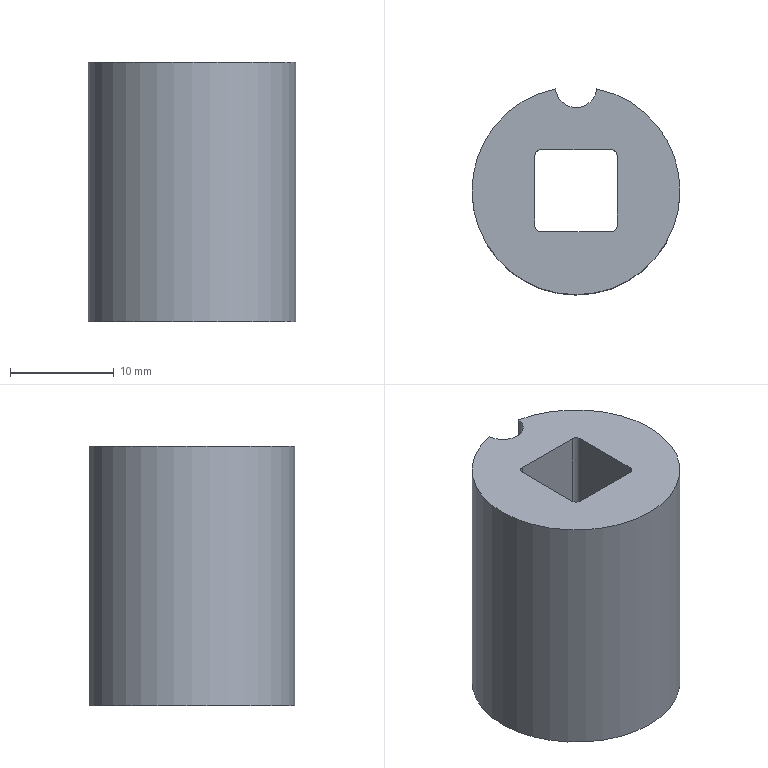Part | NX | features solid 2 | 1 solid | 14 faces | box 20 x 19.801 x 25 mm | volume 5087 mm3 | cylinder 7 | plane 7 | commonest cylinder face diameters 1.1 x4 4 x1 12.6 x1 20 x1
STEP:
#1=CARTESIAN_POINT('',(-371.503,508.125,-39.));
#2=VERTEX_POINT('',#1);
#3=CARTESIAN_POINT('',(-371.503,508.125,-14.));
#4=VERTEX_POINT('',#3);
#5=CARTESIAN_POINT('',(-371.503,508.125,-26.5));
#6=DIRECTION('',(0.,0.,1.));
#7=VECTOR('',#6,1000.);
#8=LINE('',#5,#7);
#9=EDGE_CURVE('',#2,#4,#8,.T.);
#10=ORIENTED_EDGE('',*,*,#9,.T.);
#11=CARTESIAN_POINT('',(-375.483,508.127,-14.));
#12=VERTEX_POINT('',#11);
#13=CARTESIAN_POINT('',(-373.499,498.326,-14.));
#14=DIRECTION('',(0.,0.,-1.));
#15=DIRECTION('',(0.000611,1.,0.));
#16=AXIS2_PLACEMENT_3D('',#13,#14,#15);
#17=CIRCLE('',#16,10.);
#18=EDGE_CURVE('',#4,#12,#17,.T.);
#19=ORIENTED_EDGE('',*,*,#18,.T.);
#20=CARTESIAN_POINT('',(-375.483,508.127,-39.));
#21=VERTEX_POINT('',#20);
#22=CARTESIAN_POINT('',(-375.483,508.127,-26.5));
#23=DIRECTION('',(0.,0.,1.));
#24=VECTOR('',#23,1000.);
#25=LINE('',#22,#24);
#26=EDGE_CURVE('',#12,#21,#25,.F.);
#27=ORIENTED_EDGE('',*,*,#26,.T.);
#28=CARTESIAN_POINT('',(-373.499,498.326,-39.));
#29=DIRECTION('',(0.,0.,-1.));
#30=DIRECTION('',(0.000611,1.,0.));
#31=AXIS2_PLACEMENT_3D('',#28,#29,#30);
#32=CIRCLE('',#31,10.);
#33=EDGE_CURVE('',#2,#21,#32,.T.);
#34=ORIENTED_EDGE('',*,*,#33,.F.);
#35=EDGE_LOOP('',(#10,#19,#27,#34));
#36=FACE_BOUND('',#35,.T.);
#37=CARTESIAN_POINT('',(-373.499,498.326,-39.));
#38=DIRECTION('',(0.,0.,1.));
#39=DIRECTION('',(0.000611,1.,0.));
#40=AXIS2_PLACEMENT_3D('',#37,#38,#39);
#41=CYLINDRICAL_SURFACE('',#40,10.);
#42=ADVANCED_FACE('',(#36),#41,.T.);
#43=CARTESIAN_POINT('',(-373.495,504.626,-39.));
#44=VERTEX_POINT('',#43);
#45=CARTESIAN_POINT('',(-373.499,498.326,-39.));
#46=DIRECTION('',(0.,0.,-1.));
#47=DIRECTION('',(0.000611,1.,0.));
#48=AXIS2_PLACEMENT_3D('',#45,#46,#47);
#49=CIRCLE('',#48,6.3);
#50=EDGE_CURVE('',#44,#44,#49,.T.);
#51=ORIENTED_EDGE('',*,*,#50,.F.);
#52=EDGE_LOOP('',(#51));
#53=FACE_BOUND('',#52,.T.);
#54=ORIENTED_EDGE('',*,*,#33,.T.);
#55=CARTESIAN_POINT('',(-373.493,508.326,-39.));
#56=DIRECTION('',(0.,0.,-1.));
#57=DIRECTION('',(0.000611,1.,0.));
#58=AXIS2_PLACEMENT_3D('',#55,#56,#57);
#59=CIRCLE('',#58,2.);
#60=EDGE_CURVE('',#2,#21,#59,.T.);
#61=ORIENTED_EDGE('',*,*,#60,.F.);
#62=EDGE_LOOP('',(#54,#61));
#63=FACE_BOUND('',#62,.T.);
#64=CARTESIAN_POINT('',(-373.499,498.326,-39.));
#65=DIRECTION('',(0.,0.,1.));
#66=DIRECTION('',(0.000611,1.,0.));
#67=AXIS2_PLACEMENT_3D('',#64,#65,#66);
#68=PLANE('',#67);
#69=ADVANCED_FACE('',(#53,#63),#68,.F.);
#70=CARTESIAN_POINT('',(-370.102,494.374,-14.));
#71=VERTEX_POINT('',#70);
#72=CARTESIAN_POINT('',(-376.902,494.378,-14.));
#73=VERTEX_POINT('',#72);
#74=CARTESIAN_POINT('',(-369.552,494.374,-14.));
#75=DIRECTION('',(-1.,0.000611,0.));
#76=VECTOR('',#75,1000.);
#77=LINE('',#74,#76);
#78=EDGE_CURVE('',#71,#73,#77,.T.);
#79=ORIENTED_EDGE('',*,*,#78,.T.);
#80=CARTESIAN_POINT('',(-377.451,494.928,-14.));
#81=VERTEX_POINT('',#80);
#82=CARTESIAN_POINT('',(-376.901,494.928,-14.));
#83=DIRECTION('',(0.,0.,-1.));
#84=DIRECTION('',(0.000611,1.,0.));
#85=AXIS2_PLACEMENT_3D('',#82,#83,#84);
#86=CIRCLE('',#85,0.55);
#87=EDGE_CURVE('',#81,#73,#86,.F.);
#88=ORIENTED_EDGE('',*,*,#87,.F.);
#89=CARTESIAN_POINT('',(-377.447,501.728,-14.));
#90=VERTEX_POINT('',#89);
#91=CARTESIAN_POINT('',(-377.452,494.378,-14.));
#92=DIRECTION('',(0.000611,1.,0.));
#93=VECTOR('',#92,1000.);
#94=LINE('',#91,#93);
#95=EDGE_CURVE('',#81,#90,#94,.T.);
#96=ORIENTED_EDGE('',*,*,#95,.T.);
#97=CARTESIAN_POINT('',(-376.897,502.278,-14.));
#98=VERTEX_POINT('',#97);
#99=CARTESIAN_POINT('',(-376.897,501.728,-14.));
#100=DIRECTION('',(0.,0.,-1.));
#101=DIRECTION('',(0.000611,1.,0.));
#102=AXIS2_PLACEMENT_3D('',#99,#100,#101);
#103=CIRCLE('',#102,0.55);
#104=EDGE_CURVE('',#98,#90,#103,.F.);
#105=ORIENTED_EDGE('',*,*,#104,.F.);
#106=CARTESIAN_POINT('',(-370.097,502.274,-14.));
#107=VERTEX_POINT('',#106);
#108=CARTESIAN_POINT('',(-369.547,502.274,-14.));
#109=DIRECTION('',(-1.,0.000611,0.));
#110=VECTOR('',#109,1000.);
#111=LINE('',#108,#110);
#112=EDGE_CURVE('',#107,#98,#111,.T.);
#113=ORIENTED_EDGE('',*,*,#112,.F.);
#114=CARTESIAN_POINT('',(-369.547,501.724,-14.));
#115=VERTEX_POINT('',#114);
#116=CARTESIAN_POINT('',(-370.097,501.724,-14.));
#117=DIRECTION('',(0.,0.,-1.));
#118=DIRECTION('',(0.000611,1.,0.));
#119=AXIS2_PLACEMENT_3D('',#116,#117,#118);
#120=CIRCLE('',#119,0.55);
#121=EDGE_CURVE('',#115,#107,#120,.F.);
#122=ORIENTED_EDGE('',*,*,#121,.F.);
#123=CARTESIAN_POINT('',(-369.551,494.924,-14.));
#124=VERTEX_POINT('',#123);
#125=CARTESIAN_POINT('',(-369.547,502.274,-14.));
#126=DIRECTION('',(-0.000611,-1.,0.));
#127=VECTOR('',#126,1000.);
#128=LINE('',#125,#127);
#129=EDGE_CURVE('',#115,#124,#128,.T.);
#130=ORIENTED_EDGE('',*,*,#129,.T.);
#131=CARTESIAN_POINT('',(-370.101,494.924,-14.));
#132=DIRECTION('',(0.,0.,-1.));
#133=DIRECTION('',(0.000611,1.,0.));
#134=AXIS2_PLACEMENT_3D('',#131,#132,#133);
#135=CIRCLE('',#134,0.55);
#136=EDGE_CURVE('',#71,#124,#135,.F.);
#137=ORIENTED_EDGE('',*,*,#136,.F.);
#138=EDGE_LOOP('',(#79,#88,#96,#105,#113,#122,#130,#137));
#139=FACE_BOUND('',#138,.T.);
#140=CARTESIAN_POINT('',(-373.493,508.326,-14.));
#141=DIRECTION('',(0.,0.,-1.));
#142=DIRECTION('',(0.000611,1.,0.));
#143=AXIS2_PLACEMENT_3D('',#140,#141,#142);
#144=CIRCLE('',#143,2.);
#145=EDGE_CURVE('',#4,#12,#144,.T.);
#146=ORIENTED_EDGE('',*,*,#145,.T.);
#147=ORIENTED_EDGE('',*,*,#18,.F.);
#148=EDGE_LOOP('',(#146,#147));
#149=FACE_BOUND('',#148,.T.);
#150=CARTESIAN_POINT('',(-373.499,498.326,-14.));
#151=DIRECTION('',(0.,0.,1.));
#152=DIRECTION('',(0.000611,1.,0.));
#153=AXIS2_PLACEMENT_3D('',#150,#151,#152);
#154=PLANE('',#153);
#155=ADVANCED_FACE('',(#139,#149),#154,.T.);
#156=ORIENTED_EDGE('',*,*,#50,.T.);
#157=EDGE_LOOP('',(#156));
#158=FACE_BOUND('',#157,.T.);
#159=CARTESIAN_POINT('',(-373.495,504.626,-22.));
#160=VERTEX_POINT('',#159);
#161=CARTESIAN_POINT('',(-373.499,498.326,-22.));
#162=DIRECTION('',(0.,0.,-1.));
#163=DIRECTION('',(0.000611,1.,0.));
#164=AXIS2_PLACEMENT_3D('',#161,#162,#163);
#165=CIRCLE('',#164,6.3);
#166=EDGE_CURVE('',#160,#160,#165,.T.);
#167=ORIENTED_EDGE('',*,*,#166,.F.);
#168=EDGE_LOOP('',(#167));
#169=FACE_BOUND('',#168,.T.);
#170=CARTESIAN_POINT('',(-373.499,498.326,-39.));
#171=DIRECTION('',(0.,0.,1.));
#172=DIRECTION('',(0.000611,1.,0.));
#173=AXIS2_PLACEMENT_3D('',#170,#171,#172);
#174=CYLINDRICAL_SURFACE('',#173,6.3);
#175=ADVANCED_FACE('',(#158,#169),#174,.F.);
#176=CARTESIAN_POINT('',(-370.097,502.274,-22.));
#177=VERTEX_POINT('',#176);
#178=CARTESIAN_POINT('',(-376.897,502.278,-22.));
#179=VERTEX_POINT('',#178);
#180=CARTESIAN_POINT('',(-373.497,502.276,-22.));
#181=DIRECTION('',(-1.,0.000611,0.));
#182=VECTOR('',#181,1000.);
#183=LINE('',#180,#182);
#184=EDGE_CURVE('',#177,#179,#183,.T.);
#185=ORIENTED_EDGE('',*,*,#184,.T.);
#186=CARTESIAN_POINT('',(-377.447,501.728,-22.));
#187=VERTEX_POINT('',#186);
#188=CARTESIAN_POINT('',(-376.897,501.728,-22.));
#189=DIRECTION('',(0.,0.,-1.));
#190=DIRECTION('',(0.000611,1.,0.));
#191=AXIS2_PLACEMENT_3D('',#188,#189,#190);
#192=CIRCLE('',#191,0.55);
#193=EDGE_CURVE('',#187,#179,#192,.T.);
#194=ORIENTED_EDGE('',*,*,#193,.F.);
#195=CARTESIAN_POINT('',(-377.451,494.928,-22.));
#196=VERTEX_POINT('',#195);
#197=CARTESIAN_POINT('',(-377.449,498.328,-22.));
#198=DIRECTION('',(0.000611,1.,0.));
#199=VECTOR('',#198,1000.);
#200=LINE('',#197,#199);
#201=EDGE_CURVE('',#196,#187,#200,.T.);
#202=ORIENTED_EDGE('',*,*,#201,.F.);
#203=CARTESIAN_POINT('',(-376.902,494.378,-22.));
#204=VERTEX_POINT('',#203);
#205=CARTESIAN_POINT('',(-376.901,494.928,-22.));
#206=DIRECTION('',(0.,0.,-1.));
#207=DIRECTION('',(0.000611,1.,0.));
#208=AXIS2_PLACEMENT_3D('',#205,#206,#207);
#209=CIRCLE('',#208,0.55);
#210=EDGE_CURVE('',#204,#196,#209,.T.);
#211=ORIENTED_EDGE('',*,*,#210,.F.);
#212=CARTESIAN_POINT('',(-370.102,494.374,-22.));
#213=VERTEX_POINT('',#212);
#214=CARTESIAN_POINT('',(-373.502,494.376,-22.));
#215=DIRECTION('',(-1.,0.000611,0.));
#216=VECTOR('',#215,1000.);
#217=LINE('',#214,#216);
#218=EDGE_CURVE('',#213,#204,#217,.T.);
#219=ORIENTED_EDGE('',*,*,#218,.F.);
#220=CARTESIAN_POINT('',(-369.551,494.924,-22.));
#221=VERTEX_POINT('',#220);
#222=CARTESIAN_POINT('',(-370.101,494.924,-22.));
#223=DIRECTION('',(0.,0.,-1.));
#224=DIRECTION('',(0.000611,1.,0.));
#225=AXIS2_PLACEMENT_3D('',#222,#223,#224);
#226=CIRCLE('',#225,0.55);
#227=EDGE_CURVE('',#221,#213,#226,.T.);
#228=ORIENTED_EDGE('',*,*,#227,.F.);
#229=CARTESIAN_POINT('',(-369.547,501.724,-22.));
#230=VERTEX_POINT('',#229);
#231=CARTESIAN_POINT('',(-369.549,498.324,-22.));
#232=DIRECTION('',(-0.000611,-1.,0.));
#233=VECTOR('',#232,1000.);
#234=LINE('',#231,#233);
#235=EDGE_CURVE('',#230,#221,#234,.T.);
#236=ORIENTED_EDGE('',*,*,#235,.F.);
#237=CARTESIAN_POINT('',(-370.097,501.724,-22.));
#238=DIRECTION('',(0.,0.,-1.));
#239=DIRECTION('',(0.000611,1.,0.));
#240=AXIS2_PLACEMENT_3D('',#237,#238,#239);
#241=CIRCLE('',#240,0.55);
#242=EDGE_CURVE('',#177,#230,#241,.T.);
#243=ORIENTED_EDGE('',*,*,#242,.F.);
#244=EDGE_LOOP('',(#185,#194,#202,#211,#219,#228,#236,#243));
#245=FACE_BOUND('',#244,.T.);
#246=ORIENTED_EDGE('',*,*,#166,.T.);
#247=EDGE_LOOP('',(#246));
#248=FACE_BOUND('',#247,.T.);
#249=CARTESIAN_POINT('',(-373.499,498.326,-22.));
#250=DIRECTION('',(0.,0.,1.));
#251=DIRECTION('',(0.000611,1.,0.));
#252=AXIS2_PLACEMENT_3D('',#249,#250,#251);
#253=PLANE('',#252);
#254=ADVANCED_FACE('',(#245,#248),#253,.F.);
#255=ORIENTED_EDGE('',*,*,#9,.F.);
#256=ORIENTED_EDGE('',*,*,#60,.T.);
#257=ORIENTED_EDGE('',*,*,#26,.F.);
#258=ORIENTED_EDGE('',*,*,#145,.F.);
#259=EDGE_LOOP('',(#255,#256,#257,#258));
#260=FACE_BOUND('',#259,.T.);
#261=CARTESIAN_POINT('',(-373.493,508.326,-39.));
#262=DIRECTION('',(0.,0.,1.));
#263=DIRECTION('',(0.000611,1.,0.));
#264=AXIS2_PLACEMENT_3D('',#261,#262,#263);
#265=CYLINDRICAL_SURFACE('',#264,2.);
#266=ADVANCED_FACE('',(#260),#265,.F.);
#267=ORIENTED_EDGE('',*,*,#78,.F.);
#268=CARTESIAN_POINT('',(-370.102,494.374,-14.));
#269=DIRECTION('',(0.,0.,1.));
#270=VECTOR('',#269,1000.);
#271=LINE('',#268,#270);
#272=EDGE_CURVE('',#213,#71,#271,.T.);
#273=ORIENTED_EDGE('',*,*,#272,.F.);
#274=ORIENTED_EDGE('',*,*,#218,.T.);
#275=CARTESIAN_POINT('',(-376.902,494.378,-22.));
#276=DIRECTION('',(0.,0.,1.));
#277=VECTOR('',#276,1000.);
#278=LINE('',#275,#277);
#279=EDGE_CURVE('',#73,#204,#278,.F.);
#280=ORIENTED_EDGE('',*,*,#279,.F.);
#281=EDGE_LOOP('',(#267,#273,#274,#280));
#282=FACE_BOUND('',#281,.T.);
#283=CARTESIAN_POINT('',(-369.552,494.374,-39.));
#284=DIRECTION('',(-0.000611,-1.,0.));
#285=DIRECTION('',(0.,0.,1.));
#286=AXIS2_PLACEMENT_3D('',#283,#284,#285);
#287=PLANE('',#286);
#288=ADVANCED_FACE('',(#282),#287,.F.);
#289=ORIENTED_EDGE('',*,*,#95,.F.);
#290=CARTESIAN_POINT('',(-377.451,494.928,-14.));
#291=DIRECTION('',(0.,0.,1.));
#292=VECTOR('',#291,1000.);
#293=LINE('',#290,#292);
#294=EDGE_CURVE('',#196,#81,#293,.T.);
#295=ORIENTED_EDGE('',*,*,#294,.F.);
#296=ORIENTED_EDGE('',*,*,#201,.T.);
#297=CARTESIAN_POINT('',(-377.447,501.728,-39.));
#298=DIRECTION('',(0.,0.,1.));
#299=VECTOR('',#298,1000.);
#300=LINE('',#297,#299);
#301=EDGE_CURVE('',#90,#187,#300,.F.);
#302=ORIENTED_EDGE('',*,*,#301,.F.);
#303=EDGE_LOOP('',(#289,#295,#296,#302));
#304=FACE_BOUND('',#303,.T.);
#305=CARTESIAN_POINT('',(-377.452,494.378,-39.));
#306=DIRECTION('',(-1.,0.000611,0.));
#307=DIRECTION('',(0.,0.,-1.));
#308=AXIS2_PLACEMENT_3D('',#305,#306,#307);
#309=PLANE('',#308);
#310=ADVANCED_FACE('',(#304),#309,.F.);
#311=ORIENTED_EDGE('',*,*,#112,.T.);
#312=CARTESIAN_POINT('',(-376.897,502.278,-39.));
#313=DIRECTION('',(0.,0.,1.));
#314=VECTOR('',#313,1000.);
#315=LINE('',#312,#314);
#316=EDGE_CURVE('',#179,#98,#315,.T.);
#317=ORIENTED_EDGE('',*,*,#316,.F.);
#318=ORIENTED_EDGE('',*,*,#184,.F.);
#319=CARTESIAN_POINT('',(-370.097,502.274,-39.));
#320=DIRECTION('',(0.,0.,1.));
#321=VECTOR('',#320,1000.);
#322=LINE('',#319,#321);
#323=EDGE_CURVE('',#107,#177,#322,.F.);
#324=ORIENTED_EDGE('',*,*,#323,.F.);
#325=EDGE_LOOP('',(#311,#317,#318,#324));
#326=FACE_BOUND('',#325,.T.);
#327=CARTESIAN_POINT('',(-369.547,502.274,-39.));
#328=DIRECTION('',(-0.000611,-1.,0.));
#329=DIRECTION('',(0.,0.,1.));
#330=AXIS2_PLACEMENT_3D('',#327,#328,#329);
#331=PLANE('',#330);
#332=ADVANCED_FACE('',(#326),#331,.T.);
#333=ORIENTED_EDGE('',*,*,#235,.T.);
#334=CARTESIAN_POINT('',(-369.551,494.924,-22.));
#335=DIRECTION('',(0.,0.,1.));
#336=VECTOR('',#335,1000.);
#337=LINE('',#334,#336);
#338=EDGE_CURVE('',#124,#221,#337,.F.);
#339=ORIENTED_EDGE('',*,*,#338,.F.);
#340=ORIENTED_EDGE('',*,*,#129,.F.);
#341=CARTESIAN_POINT('',(-369.547,501.724,-39.));
#342=DIRECTION('',(0.,0.,1.));
#343=VECTOR('',#342,1000.);
#344=LINE('',#341,#343);
#345=EDGE_CURVE('',#230,#115,#344,.T.);
#346=ORIENTED_EDGE('',*,*,#345,.F.);
#347=EDGE_LOOP('',(#333,#339,#340,#346));
#348=FACE_BOUND('',#347,.T.);
#349=CARTESIAN_POINT('',(-369.547,502.274,-39.));
#350=DIRECTION('',(1.,-0.000611,0.));
#351=DIRECTION('',(0.,0.,1.));
#352=AXIS2_PLACEMENT_3D('',#349,#350,#351);
#353=PLANE('',#352);
#354=ADVANCED_FACE('',(#348),#353,.F.);
#355=ORIENTED_EDGE('',*,*,#242,.T.);
#356=ORIENTED_EDGE('',*,*,#345,.T.);
#357=ORIENTED_EDGE('',*,*,#121,.T.);
#358=ORIENTED_EDGE('',*,*,#323,.T.);
#359=EDGE_LOOP('',(#355,#356,#357,#358));
#360=FACE_BOUND('',#359,.T.);
#361=CARTESIAN_POINT('',(-370.097,501.724,-39.));
#362=DIRECTION('',(0.,0.,1.));
#363=DIRECTION('',(0.000611,1.,0.));
#364=AXIS2_PLACEMENT_3D('',#361,#362,#363);
#365=CYLINDRICAL_SURFACE('',#364,0.55);
#366=ADVANCED_FACE('',(#360),#365,.F.);
#367=ORIENTED_EDGE('',*,*,#193,.T.);
#368=ORIENTED_EDGE('',*,*,#316,.T.);
#369=ORIENTED_EDGE('',*,*,#104,.T.);
#370=ORIENTED_EDGE('',*,*,#301,.T.);
#371=EDGE_LOOP('',(#367,#368,#369,#370));
#372=FACE_BOUND('',#371,.T.);
#373=CARTESIAN_POINT('',(-376.897,501.728,-39.));
#374=DIRECTION('',(0.,0.,1.));
#375=DIRECTION('',(0.000611,1.,0.));
#376=AXIS2_PLACEMENT_3D('',#373,#374,#375);
#377=CYLINDRICAL_SURFACE('',#376,0.55);
#378=ADVANCED_FACE('',(#372),#377,.F.);
#379=ORIENTED_EDGE('',*,*,#210,.T.);
#380=ORIENTED_EDGE('',*,*,#294,.T.);
#381=ORIENTED_EDGE('',*,*,#87,.T.);
#382=ORIENTED_EDGE('',*,*,#279,.T.);
#383=EDGE_LOOP('',(#379,#380,#381,#382));
#384=FACE_BOUND('',#383,.T.);
#385=CARTESIAN_POINT('',(-376.901,494.928,-39.));
#386=DIRECTION('',(0.,0.,-1.));
#387=DIRECTION('',(-0.000611,-1.,0.));
#388=AXIS2_PLACEMENT_3D('',#385,#386,#387);
#389=CYLINDRICAL_SURFACE('',#388,0.55);
#390=ADVANCED_FACE('',(#384),#389,.F.);
#391=ORIENTED_EDGE('',*,*,#227,.T.);
#392=ORIENTED_EDGE('',*,*,#272,.T.);
#393=ORIENTED_EDGE('',*,*,#136,.T.);
#394=ORIENTED_EDGE('',*,*,#338,.T.);
#395=EDGE_LOOP('',(#391,#392,#393,#394));
#396=FACE_BOUND('',#395,.T.);
#397=CARTESIAN_POINT('',(-370.101,494.924,-39.));
#398=DIRECTION('',(0.,0.,-1.));
#399=DIRECTION('',(-0.000611,-1.,0.));
#400=AXIS2_PLACEMENT_3D('',#397,#398,#399);
#401=CYLINDRICAL_SURFACE('',#400,0.55);
#402=ADVANCED_FACE('',(#396),#401,.F.);
#403=CLOSED_SHELL('',(#42,#69,#155,#175,#254,#266,#288,#310,#332,#354,#366,#378,#390,#402));
#404=MANIFOLD_SOLID_BREP('',#403);
#405=(LENGTH_UNIT()NAMED_UNIT(*)SI_UNIT(.MILLI.,.METRE.));
#406=UNCERTAINTY_MEASURE_WITH_UNIT(LENGTH_MEASURE(0.00001),#405,'','');
#407=(NAMED_UNIT(*)PLANE_ANGLE_UNIT()SI_UNIT($,.RADIAN.));
#408=(NAMED_UNIT(*)SI_UNIT($,.STERADIAN.)SOLID_ANGLE_UNIT());
#409=(GEOMETRIC_REPRESENTATION_CONTEXT(3)GLOBAL_UNCERTAINTY_ASSIGNED_CONTEXT((#406))GLOBAL_UNIT_ASSIGNED_CONTEXT((#405,#407,#408))REPRESENTATION_CONTEXT('',''));
#410=ADVANCED_BREP_SHAPE_REPRESENTATION('',(#404),#409);